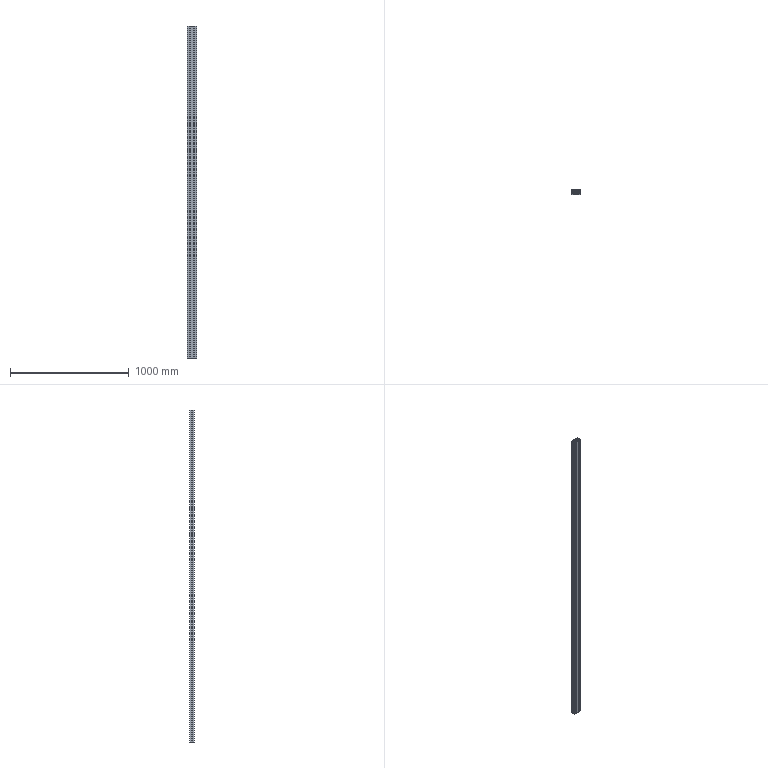Part | SolidWorks | features BaseBody 1, MoveFace 1 | 1 solid | 272 faces | box 80 x 40 x 2800 mm | volume 3366685 mm3 | plane 144 | cylinder 128 | commonest cylinder face diameters 0.4 x48 2 x48 1.998 x8 5.2 x8 1 x4 4 x4